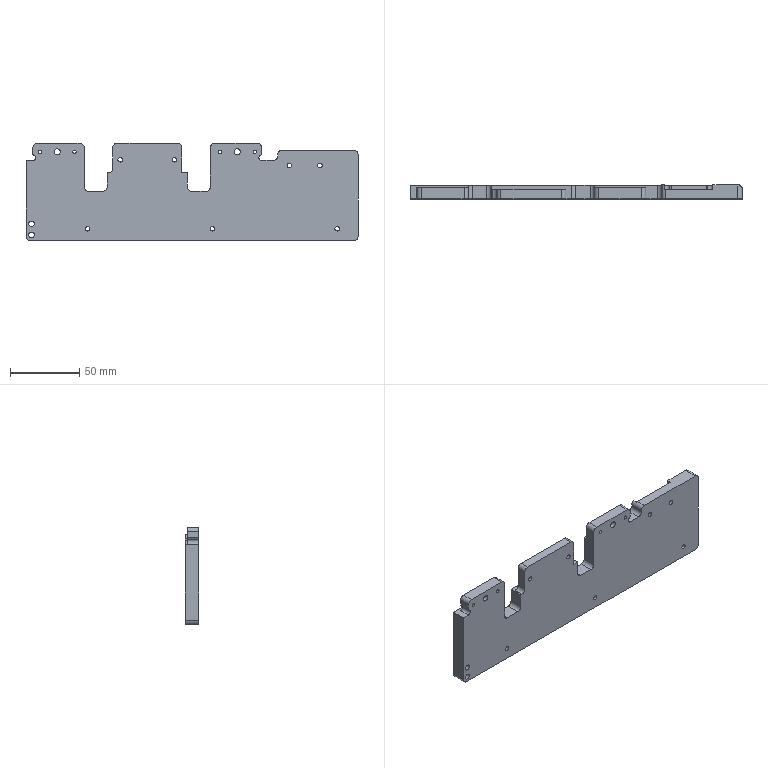CAM job | NX | 3+2 milling, drilling | part box 239.5 x 10 x 70 mm | stock box 244.5 x 12 x 75 mm
Tools:
number,name,description,diameter,corner_radius,flute_length,length,flutes
4,D4,平底铣刀-粗,4.0,0.0,25.0,75.0,2
9,D10,平底铣刀-粗,10.0,0.0,35.0,75.0,2
11,D3-J,平底铣刀-精,3.0,0.0,50.0,75.0,2
11,D4-J,平底铣刀-精,4.0,0.0,50.0,75.0,2
7,D6-J,平底铣刀-精,6.0,0.0,25.0,75.0,2
1,D80R0.8_FACEMILL,圆鼻刀-粗,80.0,0.8,50.0,75.0,2
1,D80R0.8_FACEMILL-J,圆鼻刀-精,80.0,0.8,50.0,75.0,2
2,D6_CHAMFERMILL,倒角刀,6.0,0.0,3.0,25.0,2
20,M3X0.5,丝锥,2.5,0.0,35.0,50.0,2
21,M4X0.7,丝锥,3.3,0.0,35.0,50.0,2
17,D4_REAMER,Drilling Tool,4.0,0.0,75.0,100.0,6
12,ZT2.5,钻头,2.5,0.0,35.0,50.0,2
11,ZT4.5,钻头,4.5,0.0,35.0,50.0,2
13,DRILL3.3,Twist Drill 3.3 mm,3.3,0.0,35.0,35.008,2
18,ZT3.9,Drilling Tool,3.9,0.0,35.0,50.0,2
Operations:
program,operation,operation_type,tool,method,geometry_group,spindle_rpm,surface_speed,feed_per_tooth,feed_cut,feed_plunge,cut_length_mm,path_length_mm,cut_time_min,machine_time_min
B,FLOORWALL-FACEONEPASS-ROUGH_COPY,VolumeBased25DMillingOperation,D80R0.8_FACEMILL,LAYERED-ROUGH-DEPTHK-STEPG,W-B,2800.0,703.696,0.5357,3000.0,100.0,1391.039,2456.693,0.4637,0.5702
B,FLOORWALL-FACEONEPASS-FINISH_COPY,VolumeBased25DMillingOperation,D80R0.8_FACEMILL-J,SIDEEDGE-FINISH-DEPTHK-STEPG,W-B,4000.0,1005.28,0.125,1000.0,100.0,347.563,383.563,0.3476,0.3512
B,FLOORWALL-LAYERED-ROUGH-MID_COPY,VolumeBased25DMillingOperation,D10,LAYERED-ROUGH-DEPTHK-STEPG,W-B,8000.0,251.32,0.25,4000.0,100.0,898.289,1111.306,0.2246,0.2459
B,FLOORWALL-LAYERED-ROUGH-MID_COPY_COPY,VolumeBased25DMillingOperation,D10,LAYERED-ROUGH-DEPTHK-STEPG,W-B,8000.0,251.32,0.25,4000.0,100.0,1594.494,1724.208,0.3986,0.4116
B,FLOORWALL-LAYERED-ROUGH-MID_COPY_1,VolumeBased25DMillingOperation,D10,LAYERED-ROUGH-DEPTHK-STEPG,W-B,8000.0,251.32,0.25,4000.0,100.0,706.08,761.542,0.1765,0.1821
B,CONSTZ-FINISH-ZIGZAGWALL_COPY,ZLevelMilling,D10,CONSTZ-WALL-DEPTHK-STEPG,W-B,7000.0,219.911,0.2857,4000.0,100.0,995.381,1020.623,0.2488,0.2514
B,MILL-COUNTERSINK_1,CylinderMilling,D4,METHOD,W-B,8000.0,100.531,0.1125,1800.0,100.0,376.064,602.664,0.2089,0.2316
B,MILL-HOLE_1,CylinderMilling,D4-J,METHOD,W-B,8000.0,100.531,0.0375,600.0,100.0,35.035,271.435,0.0584,0.082
B,CONSTZ-SMOOTHCORNER-D4REF10_COPY,ZLevelMilling,D4-J,LAYERED-FINISH-DEPTHK-STEPG,W-B,8000.0,100.528,0.0625,1000.0,100.0,318.781,393.812,0.3188,0.3263
B,FLOORWALL-FINISH-BOTTOM-MID_COPY_1,VolumeBased25DMillingOperation,D4-J,FINISH-STEPDEPTH-OFF,W-B,8000.0,100.528,0.05,800.0,100.0,437.289,463.895,0.5466,0.5493
B,DRILL-CHAMFER_4,Operation,D6_CHAMFERMILL,METHOD,W-B,8000.0,150.796,0.0625,1000.0,0.0,19.0,246.402,0.019,0.0417
B,DRILL-CHAMFER_5,Operation,D6_CHAMFERMILL,METHOD,W-B,8000.0,150.796,0.0625,1000.0,0.0,36.4,423.536,0.0364,0.0751
B,DRILL-CHAMFER_6,Operation,D6_CHAMFERMILL,METHOD,W-B,8000.0,150.796,0.0625,1000.0,0.0,10.6,72.744,0.0106,0.0168
B,PLANARDEBURR6X45L_COPY,SurfaceContour,D6_CHAMFERMILL,WALL_CHAMFER-DEPTH0-STEPG,W-B,6500.0,122.519,0.1154,1500.0,100.0,1035.735,2112.312,0.6905,0.7981
B,FLOORWALL-CHAMFER_COPY,VolumeBased25DMillingOperation,D6_CHAMFERMILL,WALL_CHAMFER-DEPTH0-STEPG,W-B,6500.0,122.519,0.1154,1500.0,100.0,74.44,116.84,0.0496,0.0539
B,FLOORWALL-FINISH-BOTTOM-MID_COPY,VolumeBased25DMillingOperation,D6-J,FINISH-STEPDEPTH-OFF,W-B,8000.0,251.32,0.0625,1000.0,100.0,919.374,1149.702,0.9194,0.9424
B,FLOORWALL-FINISH-SIDE-MID-SELBOTTOM_COPY,VolumeBased25DMillingOperation,D6-J,SIDEEDGE-FINISH-DEPTHK-STEPG,W-B,8000.0,251.32,0.0625,1000.0,100.0,97.451,213.657,0.0975,0.1091
B,FLOORWALL-FINISH-SIDE-MID-SELBOTTOM_COPY_1,VolumeBased25DMillingOperation,D6-J,SIDEEDGE-FINISH-DEPTHK-STEPG,W-B,8000.0,251.32,0.0625,1000.0,100.0,62.167,90.173,0.0622,0.065
B,FLOORWALL-FINISH-SIDE-MID-SELBOTTOM_COPY_2,VolumeBased25DMillingOperation,D4-J,SIDEEDGE-FINISH-DEPTHK-STEPG,W-B,8000.0,100.528,0.05,800.0,100.0,93.515,121.121,0.1169,0.1197
A,TOPFACE-ROUGH,FaceMilling,D80R0.8_FACEMILL,LAYERED-ROUGH-DEPTHK-STEPG,W-A,4000.0,1005.31,0.375,3000.0,100.0,333.5,369.3,0.1112,0.1147
A,TOPFACE,FaceMilling,D80R0.8_FACEMILL,SIDEEDGE-FINISH-DEPTHK-STEPG,W-A,4000.0,1005.31,0.125,1000.0,100.0,333.5,369.5,0.3335,0.3371
A,CAVITYMILL-ROUGH-MID_COPY,CavityMilling,D10,LAYERED-ROUGH-DEPTHK-STEPG,W-A,8000.0,251.327,0.3125,5000.0,100.0,33443.059,34002.259,6.689,6.773
A,SPOT-DEPTH0.8,Operation,D6_CHAMFERMILL,NONE,W-A,8000.0,150.796,0.0312,500.0,90.0,27.0,551.544,0.054,0.1065
A,THRUHOLE-M3TAPDRILL,Operation,ZT2.5,NONE,W-A,3000.0,23.562,0.05,300.0,90.0,59.004,316.053,0.1967,0.2224
A,THRUHOLE-M4TAPDRILL,Operation,DRILL3.3,NONE,W-A,3000.0,31.102,0.05,300.0,90.0,106.54,550.969,0.3551,0.3996
A,THRUHOLE-PRECPREDRILL4.0,Operation,ZT3.9,NONE,W-A,3000.0,36.757,0.0417,250.0,90.0,30.252,109.566,0.121,0.1289
A,THRUHOLE-5-6,Operation,ZT4.5,NONE,W-A,3000.0,42.411,0.025,150.0,90.0,15.504,202.012,0.1034,0.122
A,PROFILE-SIDE,ZLevelMilling,D3-J,METHOD,W-A,9000.0,84.823,0.1111,2000.0,80.0,3803.318,4325.134,1.903,1.955
A,SOLIDONLY,SurfaceContour,D6_CHAMFERMILL,METHOD,W-A,8000.0,150.796,0.1875,3000.0,100.0,771.564,807.365,0.2572,0.2608
A,DRILL-CHAMFER_1,Operation,D6_CHAMFERMILL,METHOD,W-A,8000.0,150.796,0.0312,500.0,0.0,19.0,242.402,0.038,0.0603
A,DRILL-CHAMFER_2,Operation,D6_CHAMFERMILL,METHOD,W-A,8000.0,150.796,0.0312,500.0,0.0,36.4,423.256,0.0728,0.1115
A,DRILL-CHAMFER_3,Operation,D6_CHAMFERMILL,METHOD,W-A,8000.0,150.796,0.0312,500.0,0.0,10.6,72.744,0.0212,0.0274
A,MILL-CHAMFER_1,PlanarMilling,D6_CHAMFERMILL,METHOD,W-A,8000.0,150.796,0.0312,500.0,100.0,34.706,247.805,0.0694,0.0907
A,THRUHOLE-TAPM3,Operation,M3X0.5,METHOD,W-A,800.0,6.283,0.0003,0.5,90.0,48.0,294.045,96.0,96.025
A,THRUHOLE-TAPM4,Operation,M4X0.7,METHOD,W-A,600.0,6.22,0.0006,0.7,90.0,85.6,509.089,122.286,122.328
A,REAM,Operation,D4_REAMER,METHOD,W-A,500.0,6.283,0.0167,50.0,0.0,24.0,97.062,0.48,0.4873
A,PROFILE-SEMIFINISH_2,VolumeBased25DMillingOperation,D6-J,METHOD,W-A,8000.0,251.327,0.0625,1000.0,100.0,771.781,830.781,0.7718,0.7777